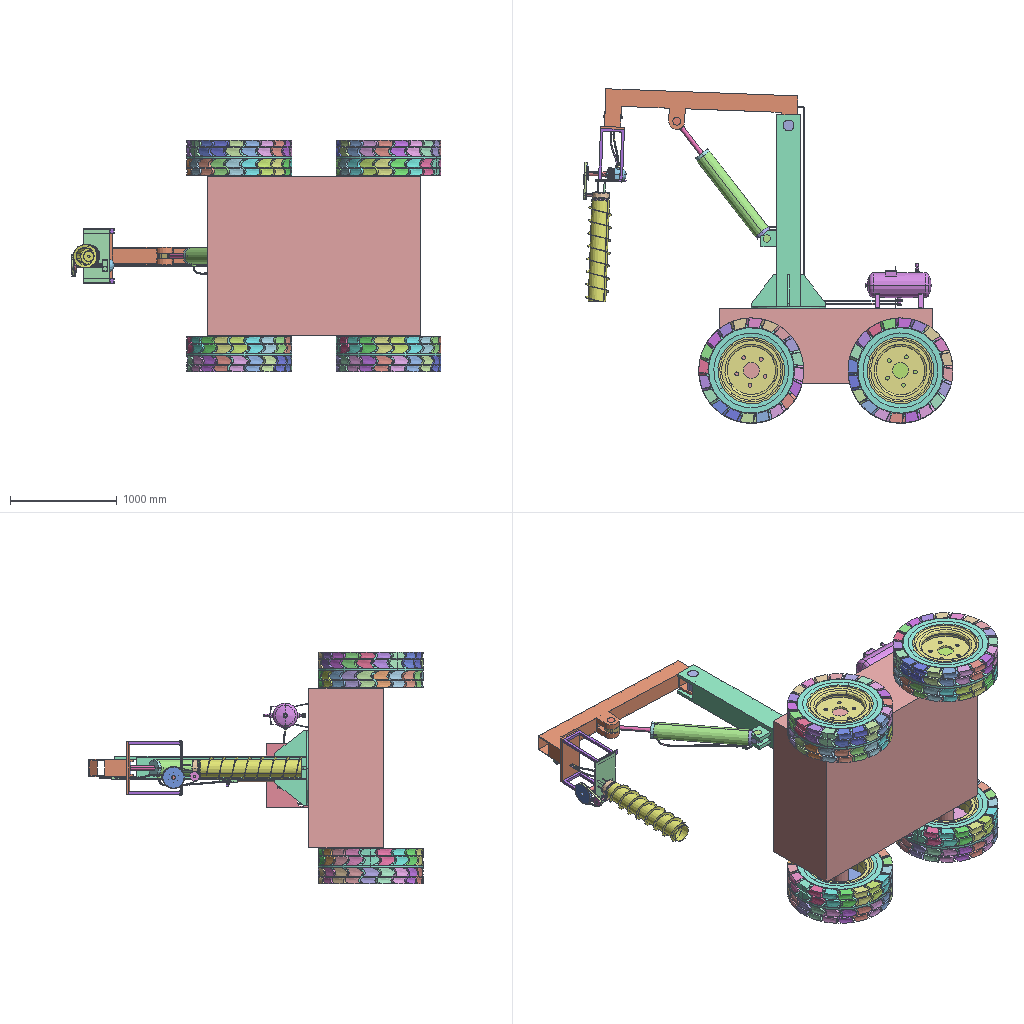Assembly | SolidWorks | 62 different items | 71 placed | box 3470 x 3136 x 2174 mm
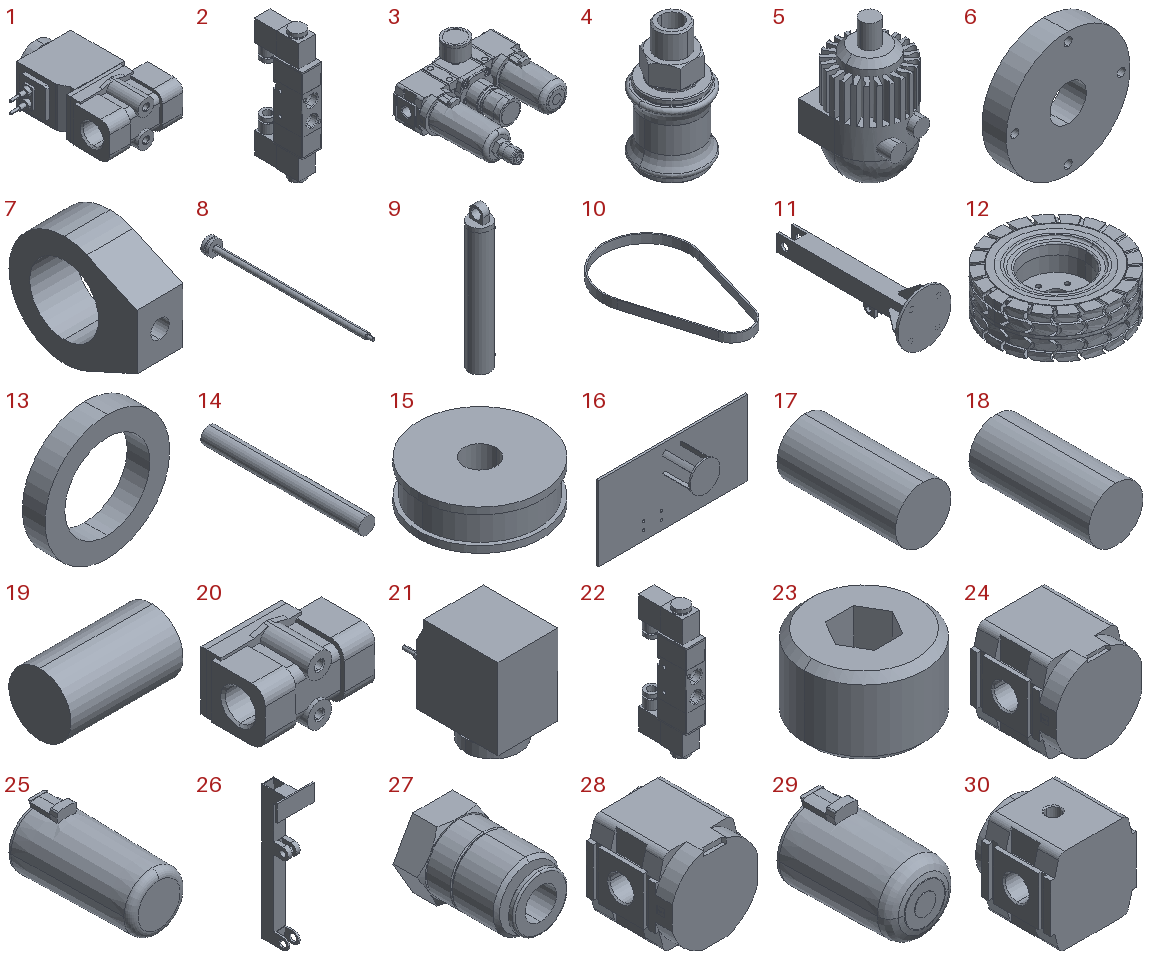Parts list (item | name | quantity | parent item | size | volume | features):
1 | (subassembly) | x1 | - | 50.5 x 61.7 x 25 mm | 39438 mm3 | features AEMSimFeature 1
2 | (subassembly) | x2 | - | 27 x 69.2 x 175.4 mm | 190277 mm3 | features AEMSimFeature 1
3 | (subassembly) | x1 | - | 167.4 x 199.6 x 104 mm | 821277 mm3 | features AEMSimFeature 1
4 | (subassembly) | x1 | - | 35.5 x 35.5 x 68.5 mm | 34573 mm3 | features AEMSimFeature 1
5 | - | x1 | - | 120 x 131 x 230 mm | 1709728 mm3 | features BaseBody 1, ICE 1
6 | - | x1 | - | 154 x 30 x 154 mm | 501657 mm3 | features BaseBody 1
7 | - | x1 | - | 50 x 139.314 x 120 mm | 424421 mm3 | features BaseBody 1
8 | - | x1 | - | 105 x 1158 x 105 mm | 1771898 mm3 | features BaseBody 1
9 | - | x1 | - | 172 x 154 x 1025 mm | 9175739 mm3 | features BaseBody 2, ICE 1
10 | - | x1 | - | 206 x 349.095 x 20 mm | 52516 mm3 | features BaseBody 1
11 | - | x1 | - | 700 x 1830 x 700 mm | 31659416 mm3 | features BaseBody 1
12 | - | x4 | - | 984.493 x 984.493 x 328 mm | 181594860 mm3 | features BaseBody 42
13 | - | x1 | - | 44 x 8 x 44 mm | 6509 mm3 | features BaseBody 1
14 | - | x1 | - | 24 x 230 x 24 mm | 104050 mm3 | features BaseBody 1
15 | - | x1 | - | 92.189 x 92.189 x 30 mm | 169612 mm3 | features BaseBody 1
16 | - | x1 | - | 500 x 114.889 x 250 mm | 1072983 mm3 | features BaseBody 1
17 | - | x1 | - | 75 x 160 x 75 mm | 706858 mm3 | features BaseBody 1
18 | - | x1 | - | 100 x 220 x 100 mm | 1727876 mm3 | features BaseBody 1
19 | - | x1 | - | 130 x 72 x 72 mm | 529296 mm3 | features BaseBody 1
20 | - | x1 | in 1 | 41 x 25.5 x 25 mm | 17055 mm3 | features BaseBody 1
21 | - | x1 | in 1 | 22.3 x 43.2 x 36.2 mm | 22382 mm3 | features BaseBody 1
22 | - | x2 | in 2 | 27 x 69.2 x 175.4 mm | 190277 mm3 | features BaseBody 1
23 | - | x1 | in 3 | 9.728 x 9.728 x 6.2 mm | 395.486 mm3 | features BaseBody 1
24 | - | x1 | in 3 | 53 x 53.5 x 53 mm | 128683 mm3 | features BaseBody 1
25 | - | x1 | in 3 | 46.4 x 94.4 x 53.2 mm | 146390 mm3 | features BaseBody 1
26 | - | x1 | - | 495 x 375.221 x 1838 mm | 21198694 mm3 | features BaseBody 1
27 | - | x1 | in 3 | 23.995 x 32.7 x 20.78 mm | 9079 mm3 | features BaseBody 1
28 | - | x1 | in 3 | 53 x 70.1 x 53 mm | 131657 mm3 | features BaseBody 1
29 | - | x1 | in 3 | 46.4 x 74.3 x 53.2 mm | 114523 mm3 | features BaseBody 1
30 | - | x1 | in 3 | 53 x 52 x 53 mm | 114626 mm3 | features BaseBody 1
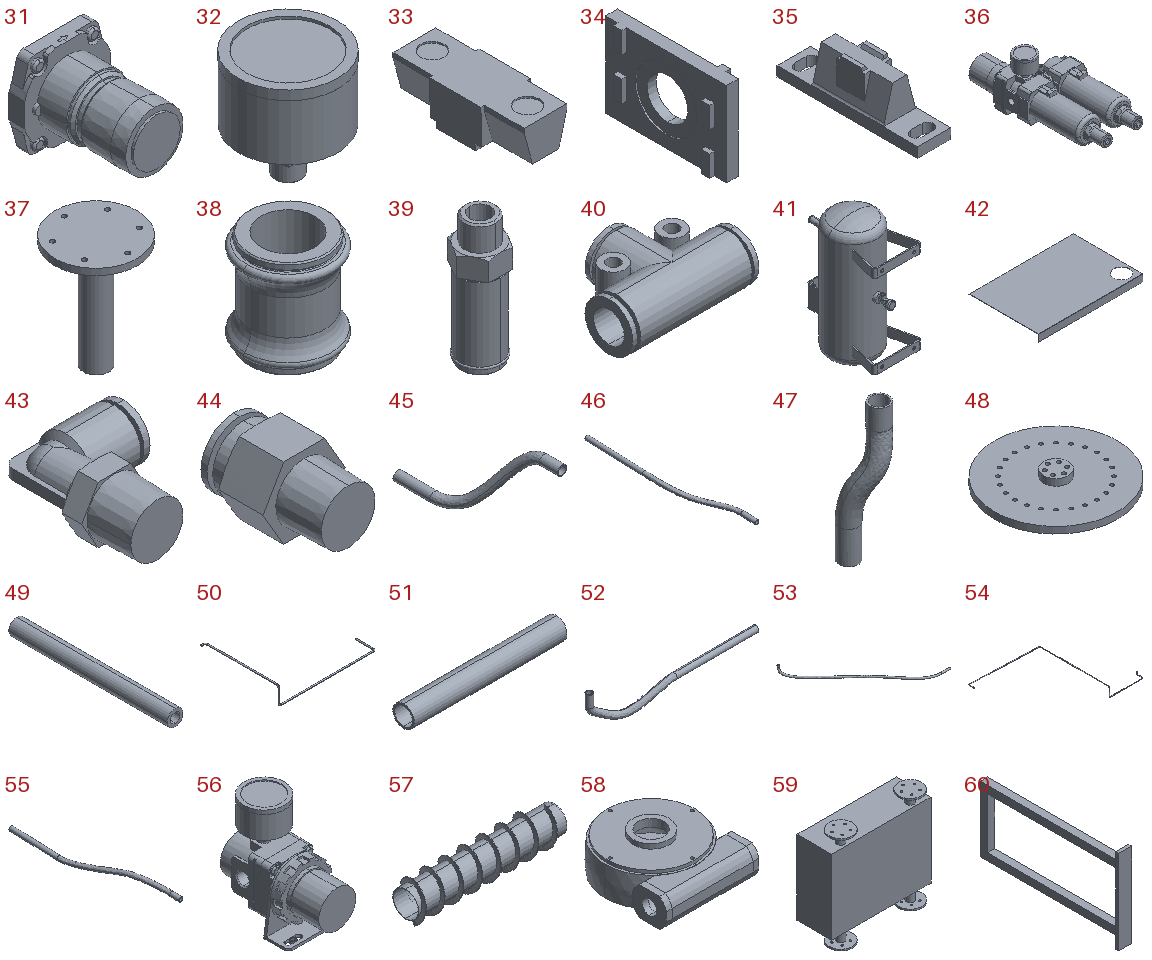31 | - | x1 | in 3 | 53 x 65 x 53 mm | 80542 mm3 | features BaseBody 1
32 | - | x1 | in 3 | 37.5 x 37.5 x 40.6 mm | 27983 mm3 | features BaseBody 1
33 | - | x2 | in 3 | 16.2 x 43 x 13.5 mm | 6701 mm3 | features BaseBody 1
34 | - | x2 | in 3 | 7.5 x 43 x 30 mm | 4813 mm3 | features BaseBody 1
35 | - | x2 | in 3 | 20 x 85 x 28 mm | 22186 mm3 | features BaseBody 1
36 | - | x1 | - | 110.2 x 240.3 x 107 mm | 709313 mm3 | features BaseBody 10
37 | - | x1 | - | 130 x 130 x 177.2 mm | 222346 mm3 | features BaseBody 1
38 | - | x1 | in 4 | 35.5 x 35.5 x 39 mm | 15226 mm3 | features BaseBody 1
39 | - | x1 | in 4 | 25.403 x 22.74 x 68.5 mm | 19347 mm3 | features BaseBody 1
40 | - | x1 | - | 41.2 x 28.55 x 15.9 mm | 7852 mm3 | features BaseBody 1
41 | - | x1 | - | 248.43 x 426.53 x 612.3 mm | 24721730 mm3 | features ICE 2, BaseBody 1, Scale 1
42 | - | x1 | - | 600 x 400 x 40 mm | 384460 mm3 | features Cut 1, EdgeFlange 1, FlatPattern 1, SMBaseFlange 1, SheetMetal 1
43 | - | x1 | - | 25.283 x 32 x 14 mm | 4555 mm3 | features BaseBody 1
44 | - | x1 | - | 19.63 x 27.3 x 17 mm | 3909 mm3 | features BaseBody 1
45 | - | x1 | - | 51.691 x 171.416 x 83.578 mm | 7159 mm3 | features 3DProfileFeature 2, Sweep 1
46 | - | x1 | - | 66.294 x 450.059 x 25.234 mm | 15866 mm3 | features 3DProfileFeature 2, Sweep 1
47 | - | x1 | - | 23 x 21.644 x 85.817 mm | 3078 mm3 | features 3DProfileFeature 2, Sweep 1
48 | - | x1 | - | 150 x 150 x 16 mm | 143087 mm3 | features BaseBody 1
49 | - | x1 | - | 10 x 100 x 10 mm | 5027 mm3 | features Extrusion 1
50 | - | x1 | - | 973.153 x 721.496 x 180.841 mm | 69029 mm3 | features 3DProfileFeature 2, Sweep 1
51 | - | x1 | - | 85.757 x 12 x 12 mm | 2964 mm3 | features 3DProfileFeature 2, Sweep 1
52 | - | x1 | - | 304.477 x 37.845 x 58.68 mm | 11725 mm3 | features 3DProfileFeature 2, Sweep 1
53 | - | x1 | - | 662.345 x 648.516 x 77.026 mm | 34265 mm3 | features 3DProfileFeature 2, Sweep 1
54 | - | x1 | - | 2689 x 1893 x 257.91 mm | 174349 mm3 | features 3DProfileFeature 2, Sweep 1
55 | - | x1 | - | 58.081 x 444.507 x 42.863 mm | 15608 mm3 | features 3DProfileFeature 2, Sweep 1
56 | - | x1 | - | - | - | features RefSurface 7, Extrusion 1
57 | - | x1 | - | 950 x 219.335 x 219.335 mm | 1959969 mm3 | features BaseBody 1
58 | - | x1 | - | 160 x 184.969 x 63 mm | 414502 mm3 | features BaseBody 4
59 | - | x1 | - | 2000 x 815 x 1960 mm | 2130497325 mm3 | features BaseBody 4
60 | - | x2 | - | 45 x 485 x 290 mm | 833625 mm3 | features BaseBody 1
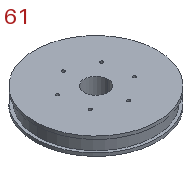61 | - | x1 | - | 210 x 210 x 30 mm | 935154 mm3 | features BaseBody 1
62 | Straight Connector KQ2H10-02AS(SMC) | x1 | - | - | - | -
Mates (type | each side: item.copy, entity, surface, feature):
Concentric | 36.1 face | 39.1 face cylinder HSV10 Body(1)
Coincident | 36.1 face | 39.1 face plane HSV10 Body(1)
Coincident | 59.1 face plane Input 1 | 42.1 face plane Edge-Flange 1
Parallel | 59.1 face plane Input 1 | 42.1 face plane Base-Flange 1
DistanceDim | 42.1 face plane Base-Flange 1 | 59.1 face plane Input 1
Coincident | 36.1 face | 42.1 face plane Base-Flange 1
Parallel | 36.1 face | 42.1 edge
Parallel | 36.1 face | 42.1 face plane Base-Flange 1
Coincident | 56.1 face plane 4-1-surface1 | 42.1 face plane Base-Flange 1
Parallel | 36.1 face | 56.1 face plane 2-1-surface1
Coincident | 11.1 face plane Input 1 | 22.1 face plane 3V320-10 By(1)
Parallel | 11.1 face plane Input 1 | 22.1 face plane 3V320-10 By(1)
Coincident | 26.1 face plane Input 1 | 22.2 face plane 3V320-10 By(1)
Parallel | 26.1 face plane Input 1 | 22.2 face plane 3V320-10 By(1)
Parallel | 56.1 face plane 2-1-surface1 | 40.1 face plane KQ2T10_00A_KQ2G
Concentric | 40.1 face cylinder KQ2T10_00A_KQ2G | 49.1 face cylinder Boss-Extrude 1
Parallel | 11.1 face plane Input 1 | 21.1 face plane 2P025-08-I - Valve Coil(1)
Concentric | 39.1 face cylinder HSV10 Body(1) | 24.1 face cylinder AF30-03-D(0)_BODY(1)
Coincident | 39.1 face plane HSV10 Body(1) | 24.1 face plane AF30-03-D(0)_BODY(1)
Coincident | 59.1 face plane Input 1 | 41.1 face plane Imported1
Parallel | 59.1 face plane Input 1 | 41.1 face plane Imported1